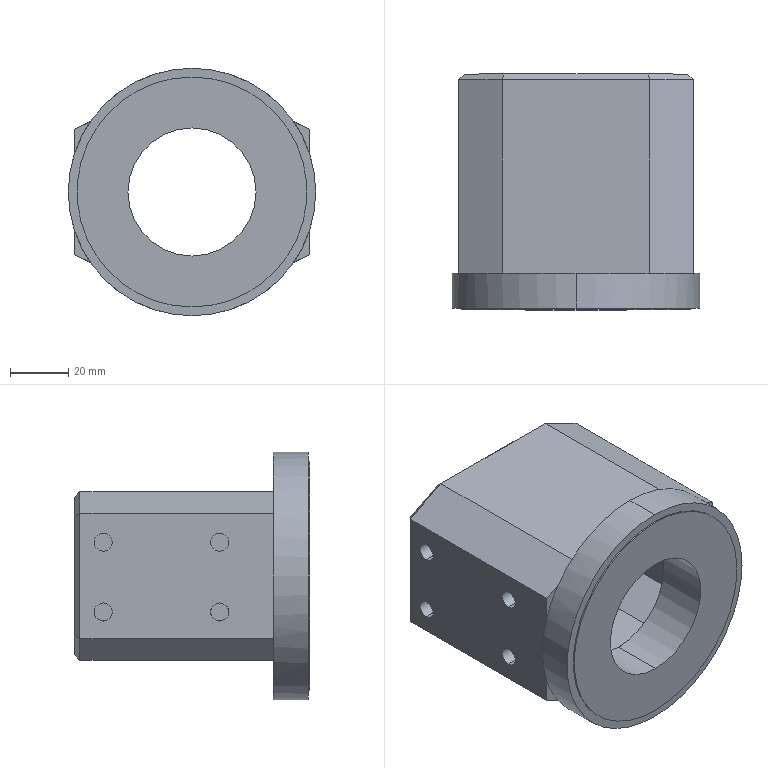Part | SolidWorks | features BaseBody 1 | 1 solid | 54 faces | box 85 x 81 x 85 mm | volume 188004 mm3 | plane 36 | cylinder 18 | commonest cylinder face diameters 6.2 x12 44 x2 79 x2 85 x2